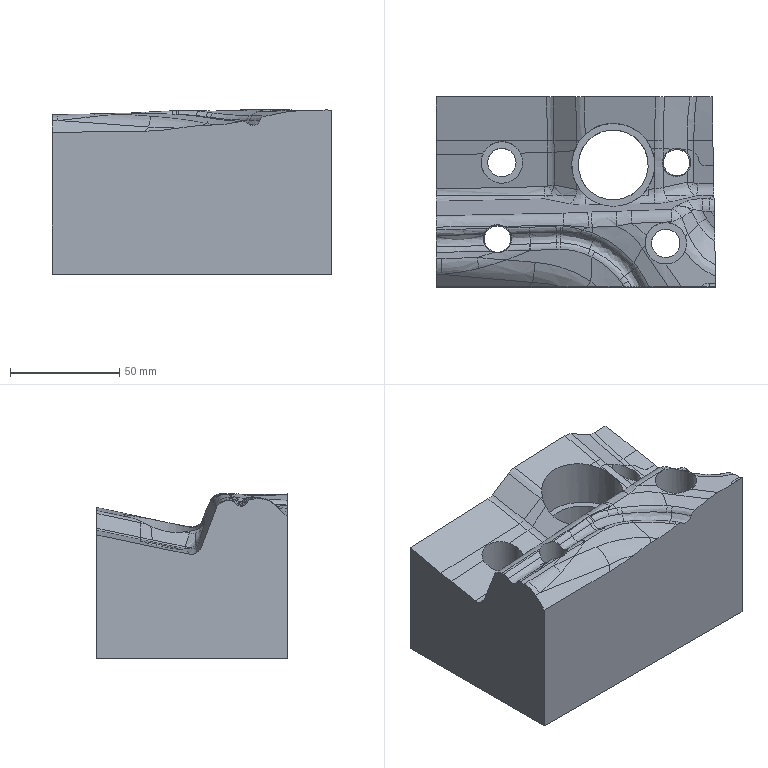Part | NX | features solid 2 | 1 solid | 151 faces | box 127.841 x 87 x 75.343 mm | volume 591848 mm3 | spline 129 | plane 11 | cylinder 11 | commonest cylinder face diameters 13 x4 12 x2 19 x2 32 x1 38 x1 41 x1